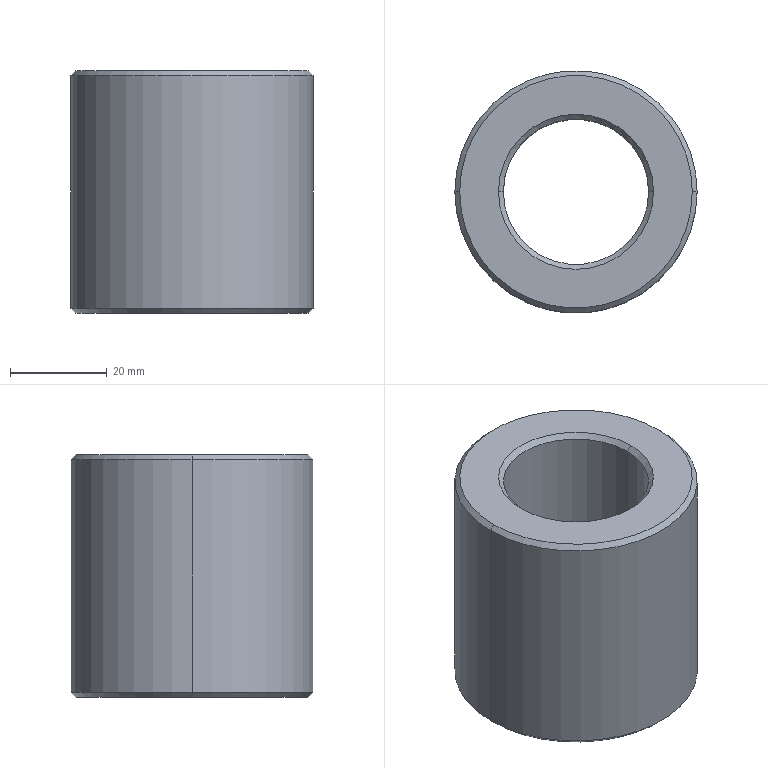Part | SolidWorks | features Chamfer 1, Extrusion 1 | 1 solid | 14 faces | box 50 x 50 x 50 mm | volume 62581 mm3 | cone 8 | cylinder 4 | plane 2 | commonest cylinder face diameters 30 x2 50 x2
STEP:
#1=CARTESIAN_POINT('',(24.,0.,50.));
#2=VERTEX_POINT('',#1);
#3=CARTESIAN_POINT('',(-24.,0.,50.));
#4=VERTEX_POINT('',#3);
#5=CARTESIAN_POINT('',(0.,0.,50.));
#6=DIRECTION('',(0.,0.,1.));
#7=DIRECTION('',(1.,0.,0.));
#8=AXIS2_PLACEMENT_3D('',#5,#6,#7);
#9=CIRCLE('',#8,24.);
#10=EDGE_CURVE('',#2,#4,#9,.T.);
#11=ORIENTED_EDGE('',*,*,#10,.F.);
#12=CARTESIAN_POINT('',(25.,0.,49.));
#13=VERTEX_POINT('',#12);
#14=CARTESIAN_POINT('',(24.,0.,50.));
#15=DIRECTION('',(0.7071,0.,-0.7071));
#16=VECTOR('',#15,1000.);
#17=LINE('',#14,#16);
#18=EDGE_CURVE('',#2,#13,#17,.T.);
#19=ORIENTED_EDGE('',*,*,#18,.T.);
#20=CARTESIAN_POINT('',(-25.,0.,49.));
#21=VERTEX_POINT('',#20);
#22=CARTESIAN_POINT('',(0.,0.,49.));
#23=DIRECTION('',(0.,0.,-1.));
#24=DIRECTION('',(1.,0.,0.));
#25=AXIS2_PLACEMENT_3D('',#22,#23,#24);
#26=CIRCLE('',#25,25.);
#27=EDGE_CURVE('',#21,#13,#26,.T.);
#28=ORIENTED_EDGE('',*,*,#27,.F.);
#29=CARTESIAN_POINT('',(-24.,0.,50.));
#30=DIRECTION('',(-0.7071,0.,-0.7071));
#31=VECTOR('',#30,1000.);
#32=LINE('',#29,#31);
#33=EDGE_CURVE('',#4,#21,#32,.T.);
#34=ORIENTED_EDGE('',*,*,#33,.F.);
#35=EDGE_LOOP('',(#11,#19,#28,#34));
#36=FACE_OUTER_BOUND('',#35,.T.);
#37=CARTESIAN_POINT('',(0.,0.,50.));
#38=DIRECTION('',(0.,0.,-1.));
#39=DIRECTION('',(-1.,0.,0.));
#40=AXIS2_PLACEMENT_3D('',#37,#38,#39);
#41=CONICAL_SURFACE('',#40,24.,0.7854);
#42=ADVANCED_FACE('',(#36),#41,.T.);
#43=CARTESIAN_POINT('',(-15.,0.,49.));
#44=VERTEX_POINT('',#43);
#45=CARTESIAN_POINT('',(15.,0.,49.));
#46=VERTEX_POINT('',#45);
#47=CARTESIAN_POINT('',(0.,0.,49.));
#48=DIRECTION('',(0.,0.,1.));
#49=DIRECTION('',(1.,0.,0.));
#50=AXIS2_PLACEMENT_3D('',#47,#48,#49);
#51=CIRCLE('',#50,15.);
#52=EDGE_CURVE('',#44,#46,#51,.T.);
#53=ORIENTED_EDGE('',*,*,#52,.F.);
#54=CARTESIAN_POINT('',(-16.,0.,50.));
#55=VERTEX_POINT('',#54);
#56=CARTESIAN_POINT('',(-15.,0.,49.));
#57=DIRECTION('',(-0.7071,0.,0.7071));
#58=VECTOR('',#57,1000.);
#59=LINE('',#56,#58);
#60=EDGE_CURVE('',#44,#55,#59,.T.);
#61=ORIENTED_EDGE('',*,*,#60,.T.);
#62=CARTESIAN_POINT('',(16.,0.,50.));
#63=VERTEX_POINT('',#62);
#64=CARTESIAN_POINT('',(0.,0.,50.));
#65=DIRECTION('',(0.,0.,-1.));
#66=DIRECTION('',(1.,0.,0.));
#67=AXIS2_PLACEMENT_3D('',#64,#65,#66);
#68=CIRCLE('',#67,16.);
#69=EDGE_CURVE('',#63,#55,#68,.T.);
#70=ORIENTED_EDGE('',*,*,#69,.F.);
#71=CARTESIAN_POINT('',(15.,0.,49.));
#72=DIRECTION('',(0.7071,0.,0.7071));
#73=VECTOR('',#72,1000.);
#74=LINE('',#71,#73);
#75=EDGE_CURVE('',#46,#63,#74,.T.);
#76=ORIENTED_EDGE('',*,*,#75,.F.);
#77=EDGE_LOOP('',(#53,#61,#70,#76));
#78=FACE_OUTER_BOUND('',#77,.T.);
#79=CARTESIAN_POINT('',(0.,0.,49.));
#80=DIRECTION('',(0.,0.,1.));
#81=DIRECTION('',(1.,0.,0.));
#82=AXIS2_PLACEMENT_3D('',#79,#80,#81);
#83=CONICAL_SURFACE('',#82,15.,0.7854);
#84=ADVANCED_FACE('',(#78),#83,.F.);
#85=CARTESIAN_POINT('',(-24.,0.,0.));
#86=VERTEX_POINT('',#85);
#87=CARTESIAN_POINT('',(24.,0.,0.));
#88=VERTEX_POINT('',#87);
#89=CARTESIAN_POINT('',(0.,0.,0.));
#90=DIRECTION('',(0.,0.,-1.));
#91=DIRECTION('',(1.,0.,0.));
#92=AXIS2_PLACEMENT_3D('',#89,#90,#91);
#93=CIRCLE('',#92,24.);
#94=EDGE_CURVE('',#86,#88,#93,.T.);
#95=ORIENTED_EDGE('',*,*,#94,.F.);
#96=CARTESIAN_POINT('',(-25.,0.,1.));
#97=VERTEX_POINT('',#96);
#98=CARTESIAN_POINT('',(-25.,0.,1.));
#99=DIRECTION('',(-0.7071,0.,0.7071));
#100=VECTOR('',#99,1000.);
#101=LINE('',#98,#100);
#102=EDGE_CURVE('',#86,#97,#101,.T.);
#103=ORIENTED_EDGE('',*,*,#102,.T.);
#104=CARTESIAN_POINT('',(25.,0.,1.));
#105=VERTEX_POINT('',#104);
#106=CARTESIAN_POINT('',(0.,0.,1.));
#107=DIRECTION('',(0.,0.,1.));
#108=DIRECTION('',(1.,0.,0.));
#109=AXIS2_PLACEMENT_3D('',#106,#107,#108);
#110=CIRCLE('',#109,25.);
#111=EDGE_CURVE('',#105,#97,#110,.T.);
#112=ORIENTED_EDGE('',*,*,#111,.F.);
#113=CARTESIAN_POINT('',(25.,0.,1.));
#114=DIRECTION('',(0.7071,0.,0.7071));
#115=VECTOR('',#114,1000.);
#116=LINE('',#113,#115);
#117=EDGE_CURVE('',#88,#105,#116,.T.);
#118=ORIENTED_EDGE('',*,*,#117,.F.);
#119=EDGE_LOOP('',(#95,#103,#112,#118));
#120=FACE_OUTER_BOUND('',#119,.T.);
#121=CARTESIAN_POINT('',(0.,0.,1.));
#122=DIRECTION('',(0.,0.,1.));
#123=DIRECTION('',(1.,0.,0.));
#124=AXIS2_PLACEMENT_3D('',#121,#122,#123);
#125=CONICAL_SURFACE('',#124,25.,0.7854);
#126=ADVANCED_FACE('',(#120),#125,.T.);
#127=CARTESIAN_POINT('',(15.,0.,1.));
#128=VERTEX_POINT('',#127);
#129=CARTESIAN_POINT('',(-15.,0.,1.));
#130=VERTEX_POINT('',#129);
#131=CARTESIAN_POINT('',(0.,0.,1.));
#132=DIRECTION('',(0.,0.,-1.));
#133=DIRECTION('',(1.,0.,0.));
#134=AXIS2_PLACEMENT_3D('',#131,#132,#133);
#135=CIRCLE('',#134,15.);
#136=EDGE_CURVE('',#128,#130,#135,.T.);
#137=ORIENTED_EDGE('',*,*,#136,.F.);
#138=CARTESIAN_POINT('',(16.,0.,0.));
#139=VERTEX_POINT('',#138);
#140=CARTESIAN_POINT('',(16.,0.,0.));
#141=DIRECTION('',(0.7071,0.,-0.7071));
#142=VECTOR('',#141,1000.);
#143=LINE('',#140,#142);
#144=EDGE_CURVE('',#128,#139,#143,.T.);
#145=ORIENTED_EDGE('',*,*,#144,.T.);
#146=CARTESIAN_POINT('',(-16.,0.,0.));
#147=VERTEX_POINT('',#146);
#148=CARTESIAN_POINT('',(0.,0.,0.));
#149=DIRECTION('',(0.,0.,1.));
#150=DIRECTION('',(1.,0.,0.));
#151=AXIS2_PLACEMENT_3D('',#148,#149,#150);
#152=CIRCLE('',#151,16.);
#153=EDGE_CURVE('',#147,#139,#152,.T.);
#154=ORIENTED_EDGE('',*,*,#153,.F.);
#155=CARTESIAN_POINT('',(-16.,0.,0.));
#156=DIRECTION('',(-0.7071,0.,-0.7071));
#157=VECTOR('',#156,1000.);
#158=LINE('',#155,#157);
#159=EDGE_CURVE('',#130,#147,#158,.T.);
#160=ORIENTED_EDGE('',*,*,#159,.F.);
#161=EDGE_LOOP('',(#137,#145,#154,#160));
#162=FACE_OUTER_BOUND('',#161,.T.);
#163=CARTESIAN_POINT('',(0.,0.,0.));
#164=DIRECTION('',(0.,0.,-1.));
#165=DIRECTION('',(-1.,0.,0.));
#166=AXIS2_PLACEMENT_3D('',#163,#164,#165);
#167=CONICAL_SURFACE('',#166,16.,0.7854);
#168=ADVANCED_FACE('',(#162),#167,.F.);
#169=ORIENTED_EDGE('',*,*,#52,.T.);
#170=CARTESIAN_POINT('',(15.,0.,50.));
#171=DIRECTION('',(0.,0.,-1.));
#172=VECTOR('',#171,1000.);
#173=LINE('',#170,#172);
#174=EDGE_CURVE('',#46,#128,#173,.T.);
#175=ORIENTED_EDGE('',*,*,#174,.T.);
#176=ORIENTED_EDGE('',*,*,#136,.T.);
#177=CARTESIAN_POINT('',(-15.,0.,50.));
#178=DIRECTION('',(0.,0.,-1.));
#179=VECTOR('',#178,1000.);
#180=LINE('',#177,#179);
#181=EDGE_CURVE('',#44,#130,#180,.T.);
#182=ORIENTED_EDGE('',*,*,#181,.F.);
#183=EDGE_LOOP('',(#169,#175,#176,#182));
#184=FACE_OUTER_BOUND('',#183,.T.);
#185=CARTESIAN_POINT('',(0.,0.,50.));
#186=DIRECTION('',(0.,0.,-1.));
#187=DIRECTION('',(-1.,0.,0.));
#188=AXIS2_PLACEMENT_3D('',#185,#186,#187);
#189=CYLINDRICAL_SURFACE('',#188,15.);
#190=ADVANCED_FACE('',(#184),#189,.F.);
#191=ORIENTED_EDGE('',*,*,#27,.T.);
#192=CARTESIAN_POINT('',(25.,0.,50.));
#193=DIRECTION('',(0.,0.,-1.));
#194=VECTOR('',#193,1000.);
#195=LINE('',#192,#194);
#196=EDGE_CURVE('',#13,#105,#195,.T.);
#197=ORIENTED_EDGE('',*,*,#196,.T.);
#198=ORIENTED_EDGE('',*,*,#111,.T.);
#199=CARTESIAN_POINT('',(-25.,0.,50.));
#200=DIRECTION('',(0.,0.,-1.));
#201=VECTOR('',#200,1000.);
#202=LINE('',#199,#201);
#203=EDGE_CURVE('',#21,#97,#202,.T.);
#204=ORIENTED_EDGE('',*,*,#203,.F.);
#205=EDGE_LOOP('',(#191,#197,#198,#204));
#206=FACE_OUTER_BOUND('',#205,.T.);
#207=CARTESIAN_POINT('',(0.,0.,50.));
#208=DIRECTION('',(0.,0.,-1.));
#209=DIRECTION('',(-1.,0.,0.));
#210=AXIS2_PLACEMENT_3D('',#207,#208,#209);
#211=CYLINDRICAL_SURFACE('',#210,25.);
#212=ADVANCED_FACE('',(#206),#211,.T.);
#213=ORIENTED_EDGE('',*,*,#69,.T.);
#214=CARTESIAN_POINT('',(0.,0.,50.));
#215=DIRECTION('',(0.,0.,-1.));
#216=DIRECTION('',(1.,0.,0.));
#217=AXIS2_PLACEMENT_3D('',#214,#215,#216);
#218=CIRCLE('',#217,16.);
#219=EDGE_CURVE('',#55,#63,#218,.T.);
#220=ORIENTED_EDGE('',*,*,#219,.T.);
#221=EDGE_LOOP('',(#213,#220));
#222=FACE_BOUND('',#221,.T.);
#223=CARTESIAN_POINT('',(0.,0.,50.));
#224=DIRECTION('',(0.,0.,1.));
#225=DIRECTION('',(1.,0.,0.));
#226=AXIS2_PLACEMENT_3D('',#223,#224,#225);
#227=CIRCLE('',#226,24.);
#228=EDGE_CURVE('',#4,#2,#227,.T.);
#229=ORIENTED_EDGE('',*,*,#228,.T.);
#230=ORIENTED_EDGE('',*,*,#10,.T.);
#231=EDGE_LOOP('',(#229,#230));
#232=FACE_OUTER_BOUND('',#231,.T.);
#233=CARTESIAN_POINT('',(0.,0.,50.));
#234=DIRECTION('',(0.,0.,1.));
#235=DIRECTION('',(1.,0.,0.));
#236=AXIS2_PLACEMENT_3D('',#233,#234,#235);
#237=PLANE('',#236);
#238=ADVANCED_FACE('',(#222,#232),#237,.T.);
#239=ORIENTED_EDGE('',*,*,#153,.T.);
#240=CARTESIAN_POINT('',(0.,0.,0.));
#241=DIRECTION('',(0.,0.,1.));
#242=DIRECTION('',(1.,0.,0.));
#243=AXIS2_PLACEMENT_3D('',#240,#241,#242);
#244=CIRCLE('',#243,16.);
#245=EDGE_CURVE('',#139,#147,#244,.T.);
#246=ORIENTED_EDGE('',*,*,#245,.T.);
#247=EDGE_LOOP('',(#239,#246));
#248=FACE_BOUND('',#247,.T.);
#249=CARTESIAN_POINT('',(0.,0.,0.));
#250=DIRECTION('',(0.,0.,-1.));
#251=DIRECTION('',(1.,0.,0.));
#252=AXIS2_PLACEMENT_3D('',#249,#250,#251);
#253=CIRCLE('',#252,24.);
#254=EDGE_CURVE('',#88,#86,#253,.T.);
#255=ORIENTED_EDGE('',*,*,#254,.T.);
#256=ORIENTED_EDGE('',*,*,#94,.T.);
#257=EDGE_LOOP('',(#255,#256));
#258=FACE_OUTER_BOUND('',#257,.T.);
#259=CARTESIAN_POINT('',(0.,0.,0.));
#260=DIRECTION('',(0.,0.,1.));
#261=DIRECTION('',(1.,0.,0.));
#262=AXIS2_PLACEMENT_3D('',#259,#260,#261);
#263=PLANE('',#262);
#264=ADVANCED_FACE('',(#248,#258),#263,.F.);
#265=ORIENTED_EDGE('',*,*,#196,.F.);
#266=CARTESIAN_POINT('',(0.,0.,49.));
#267=DIRECTION('',(0.,0.,-1.));
#268=DIRECTION('',(1.,0.,0.));
#269=AXIS2_PLACEMENT_3D('',#266,#267,#268);
#270=CIRCLE('',#269,25.);
#271=EDGE_CURVE('',#13,#21,#270,.T.);
#272=ORIENTED_EDGE('',*,*,#271,.T.);
#273=ORIENTED_EDGE('',*,*,#203,.T.);
#274=CARTESIAN_POINT('',(0.,0.,1.));
#275=DIRECTION('',(0.,0.,1.));
#276=DIRECTION('',(1.,0.,0.));
#277=AXIS2_PLACEMENT_3D('',#274,#275,#276);
#278=CIRCLE('',#277,25.);
#279=EDGE_CURVE('',#97,#105,#278,.T.);
#280=ORIENTED_EDGE('',*,*,#279,.T.);
#281=EDGE_LOOP('',(#265,#272,#273,#280));
#282=FACE_OUTER_BOUND('',#281,.T.);
#283=CARTESIAN_POINT('',(0.,0.,50.));
#284=DIRECTION('',(0.,0.,-1.));
#285=DIRECTION('',(-1.,0.,0.));
#286=AXIS2_PLACEMENT_3D('',#283,#284,#285);
#287=CYLINDRICAL_SURFACE('',#286,25.);
#288=ADVANCED_FACE('',(#282),#287,.T.);
#289=ORIENTED_EDGE('',*,*,#174,.F.);
#290=CARTESIAN_POINT('',(0.,0.,49.));
#291=DIRECTION('',(0.,0.,1.));
#292=DIRECTION('',(1.,0.,0.));
#293=AXIS2_PLACEMENT_3D('',#290,#291,#292);
#294=CIRCLE('',#293,15.);
#295=EDGE_CURVE('',#46,#44,#294,.T.);
#296=ORIENTED_EDGE('',*,*,#295,.T.);
#297=ORIENTED_EDGE('',*,*,#181,.T.);
#298=CARTESIAN_POINT('',(0.,0.,1.));
#299=DIRECTION('',(0.,0.,-1.));
#300=DIRECTION('',(1.,0.,0.));
#301=AXIS2_PLACEMENT_3D('',#298,#299,#300);
#302=CIRCLE('',#301,15.);
#303=EDGE_CURVE('',#130,#128,#302,.T.);
#304=ORIENTED_EDGE('',*,*,#303,.T.);
#305=EDGE_LOOP('',(#289,#296,#297,#304));
#306=FACE_OUTER_BOUND('',#305,.T.);
#307=CARTESIAN_POINT('',(0.,0.,50.));
#308=DIRECTION('',(0.,0.,-1.));
#309=DIRECTION('',(-1.,0.,0.));
#310=AXIS2_PLACEMENT_3D('',#307,#308,#309);
#311=CYLINDRICAL_SURFACE('',#310,15.);
#312=ADVANCED_FACE('',(#306),#311,.F.);
#313=ORIENTED_EDGE('',*,*,#144,.F.);
#314=ORIENTED_EDGE('',*,*,#303,.F.);
#315=ORIENTED_EDGE('',*,*,#159,.T.);
#316=ORIENTED_EDGE('',*,*,#245,.F.);
#317=EDGE_LOOP('',(#313,#314,#315,#316));
#318=FACE_OUTER_BOUND('',#317,.T.);
#319=CARTESIAN_POINT('',(0.,0.,0.));
#320=DIRECTION('',(0.,0.,-1.));
#321=DIRECTION('',(-1.,0.,0.));
#322=AXIS2_PLACEMENT_3D('',#319,#320,#321);
#323=CONICAL_SURFACE('',#322,16.,0.7854);
#324=ADVANCED_FACE('',(#318),#323,.F.);
#325=ORIENTED_EDGE('',*,*,#102,.F.);
#326=ORIENTED_EDGE('',*,*,#254,.F.);
#327=ORIENTED_EDGE('',*,*,#117,.T.);
#328=ORIENTED_EDGE('',*,*,#279,.F.);
#329=EDGE_LOOP('',(#325,#326,#327,#328));
#330=FACE_OUTER_BOUND('',#329,.T.);
#331=CARTESIAN_POINT('',(0.,0.,1.));
#332=DIRECTION('',(0.,0.,1.));
#333=DIRECTION('',(1.,0.,0.));
#334=AXIS2_PLACEMENT_3D('',#331,#332,#333);
#335=CONICAL_SURFACE('',#334,25.,0.7854);
#336=ADVANCED_FACE('',(#330),#335,.T.);
#337=ORIENTED_EDGE('',*,*,#60,.F.);
#338=ORIENTED_EDGE('',*,*,#295,.F.);
#339=ORIENTED_EDGE('',*,*,#75,.T.);
#340=ORIENTED_EDGE('',*,*,#219,.F.);
#341=EDGE_LOOP('',(#337,#338,#339,#340));
#342=FACE_OUTER_BOUND('',#341,.T.);
#343=CARTESIAN_POINT('',(0.,0.,49.));
#344=DIRECTION('',(0.,0.,1.));
#345=DIRECTION('',(1.,0.,0.));
#346=AXIS2_PLACEMENT_3D('',#343,#344,#345);
#347=CONICAL_SURFACE('',#346,15.,0.7854);
#348=ADVANCED_FACE('',(#342),#347,.F.);
#349=ORIENTED_EDGE('',*,*,#18,.F.);
#350=ORIENTED_EDGE('',*,*,#228,.F.);
#351=ORIENTED_EDGE('',*,*,#33,.T.);
#352=ORIENTED_EDGE('',*,*,#271,.F.);
#353=EDGE_LOOP('',(#349,#350,#351,#352));
#354=FACE_OUTER_BOUND('',#353,.T.);
#355=CARTESIAN_POINT('',(0.,0.,50.));
#356=DIRECTION('',(0.,0.,-1.));
#357=DIRECTION('',(-1.,0.,0.));
#358=AXIS2_PLACEMENT_3D('',#355,#356,#357);
#359=CONICAL_SURFACE('',#358,24.,0.7854);
#360=ADVANCED_FACE('',(#354),#359,.T.);
#361=CLOSED_SHELL('',(#42,#84,#126,#168,#190,#212,#238,#264,#288,#312,#324,#336,#348,#360));
#362=MANIFOLD_SOLID_BREP('',#361);
#363=CARTESIAN_POINT('',(0.,0.,0.));
#364=DIRECTION('',(0.,0.,1.));
#365=DIRECTION('',(1.,0.,0.));
#366=AXIS2_PLACEMENT_3D('',#363,#364,#365);
#367=(LENGTH_UNIT()NAMED_UNIT(*)SI_UNIT(.MILLI.,.METRE.));
#368=UNCERTAINTY_MEASURE_WITH_UNIT(LENGTH_MEASURE(0.00001),#367,'','');
#369=(NAMED_UNIT(*)PLANE_ANGLE_UNIT()SI_UNIT($,.RADIAN.));
#370=(NAMED_UNIT(*)SI_UNIT($,.STERADIAN.)SOLID_ANGLE_UNIT());
#371=(GEOMETRIC_REPRESENTATION_CONTEXT(3)GLOBAL_UNCERTAINTY_ASSIGNED_CONTEXT((#368))GLOBAL_UNIT_ASSIGNED_CONTEXT((#367,#369,#370))REPRESENTATION_CONTEXT('',''));
#372=ADVANCED_BREP_SHAPE_REPRESENTATION('',(#362,#366),#371);